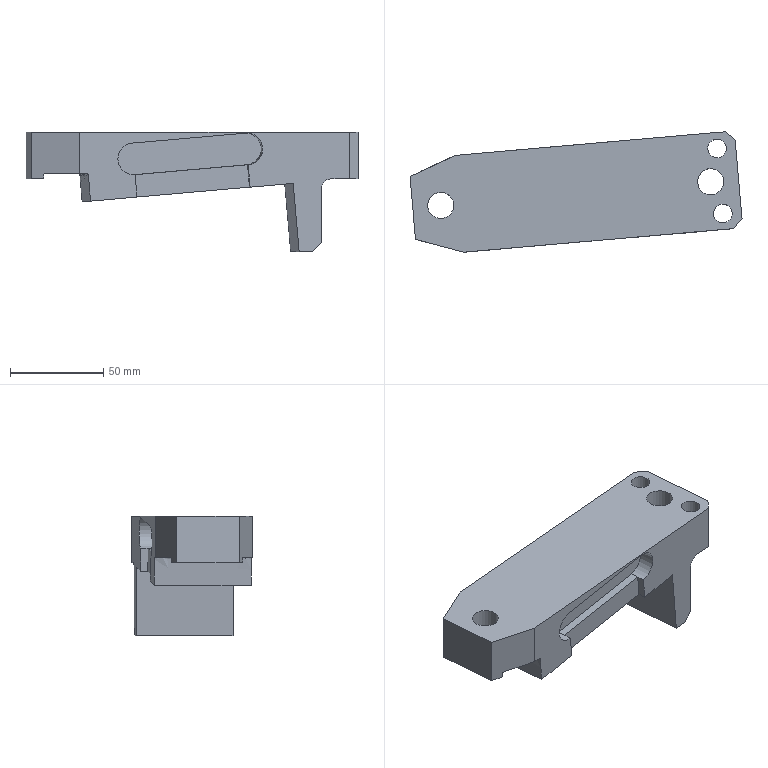Part | NX | features solid 2 | 1 solid | 49 faces | box 177.637 x 64.44 x 64.002 mm | volume 246023 mm3 | plane 34 | cylinder 14 | spline 1 | commonest cylinder face diameters 10 x4 17 x4 11 x2 14 x2 20 x2